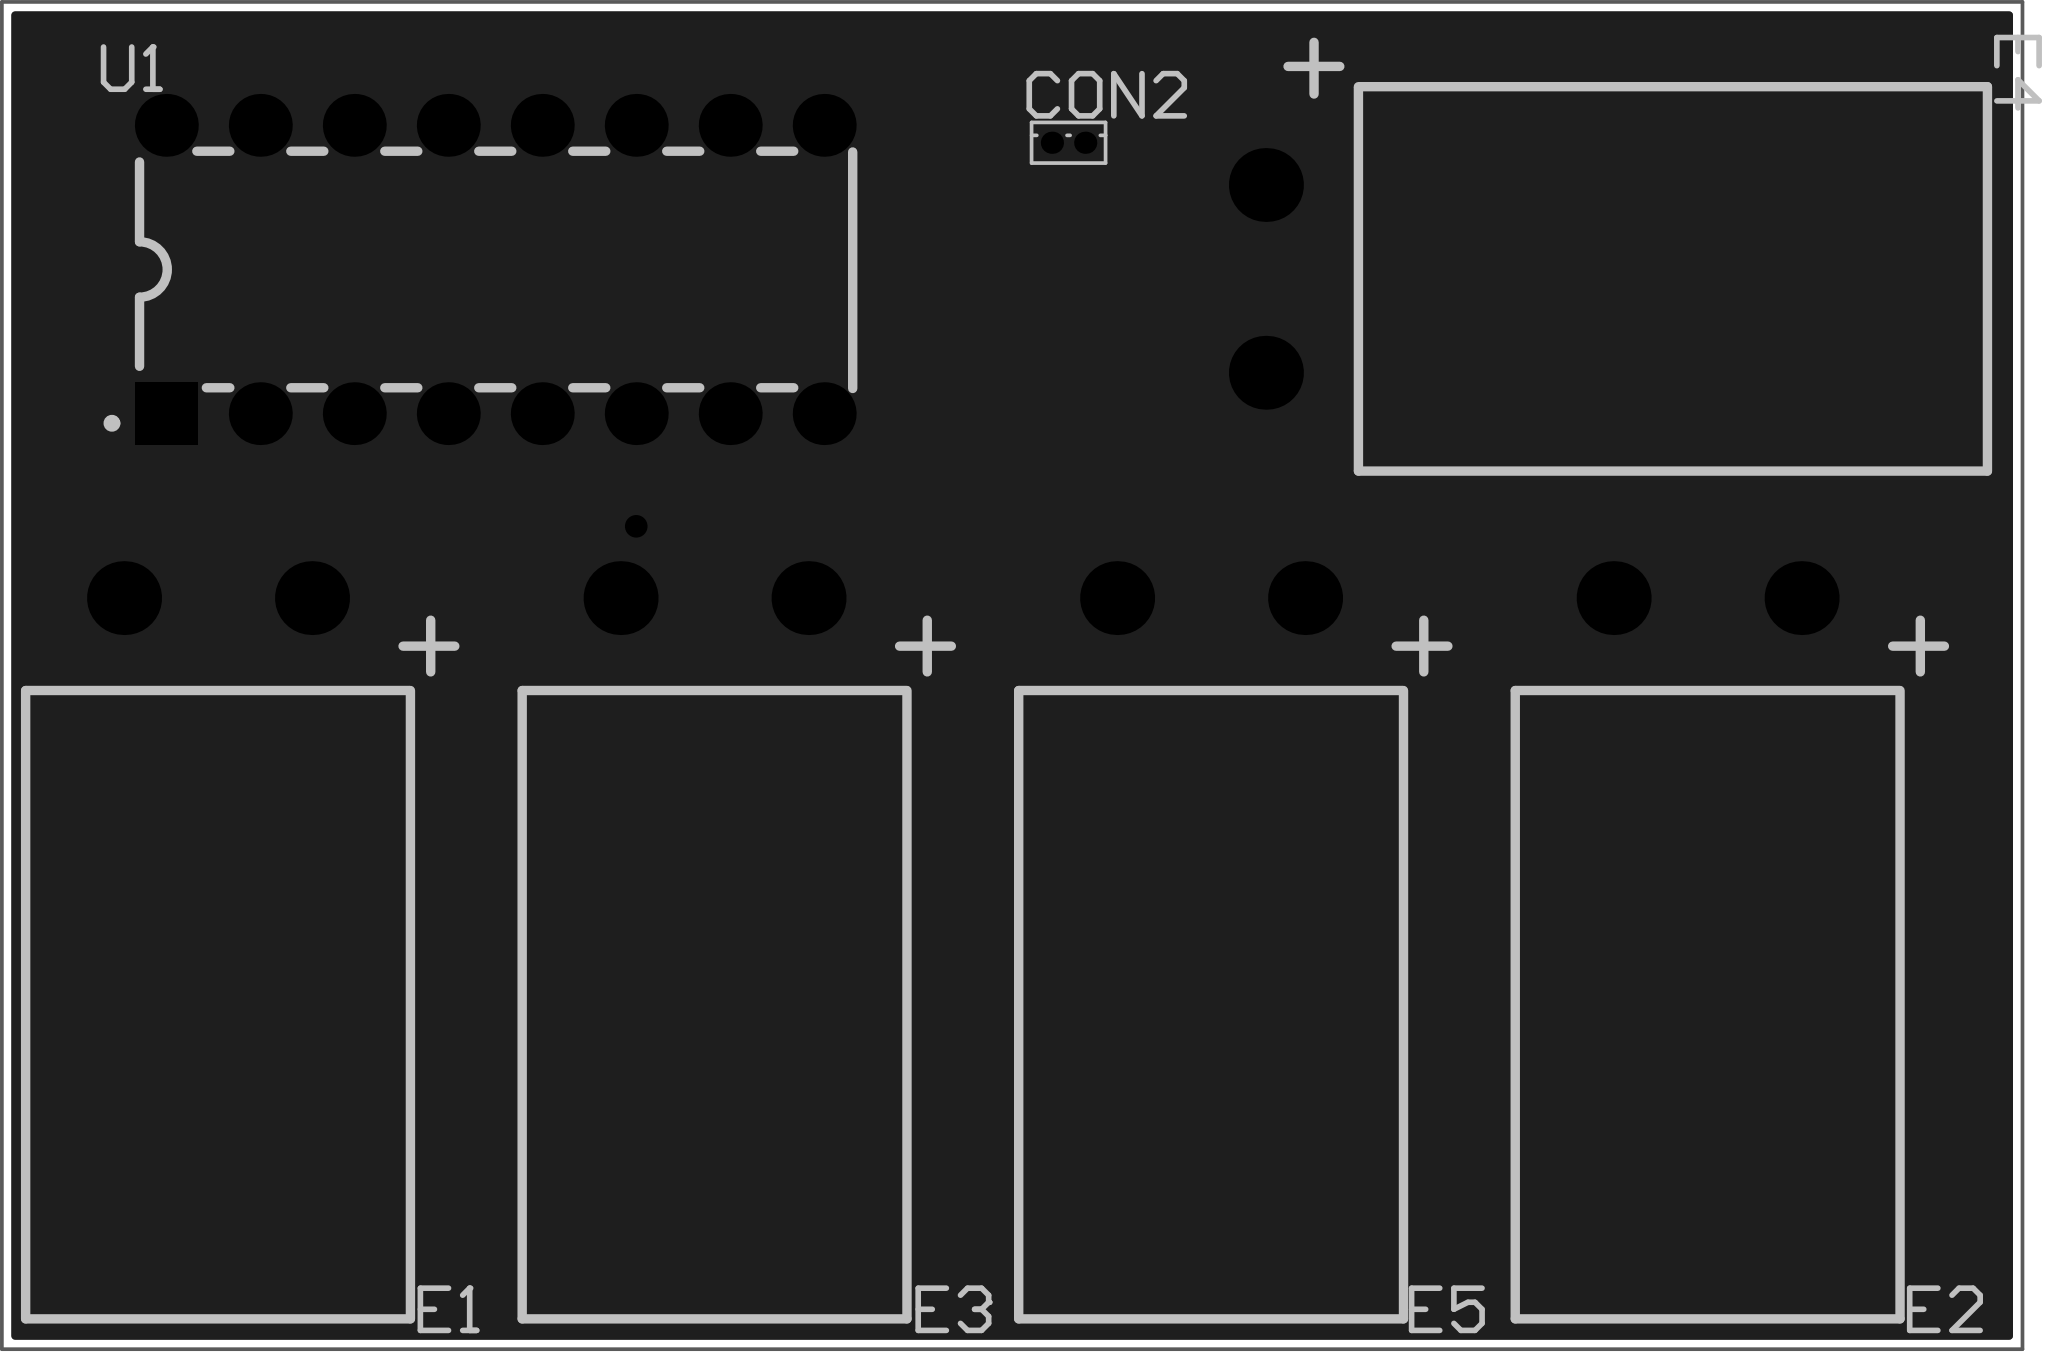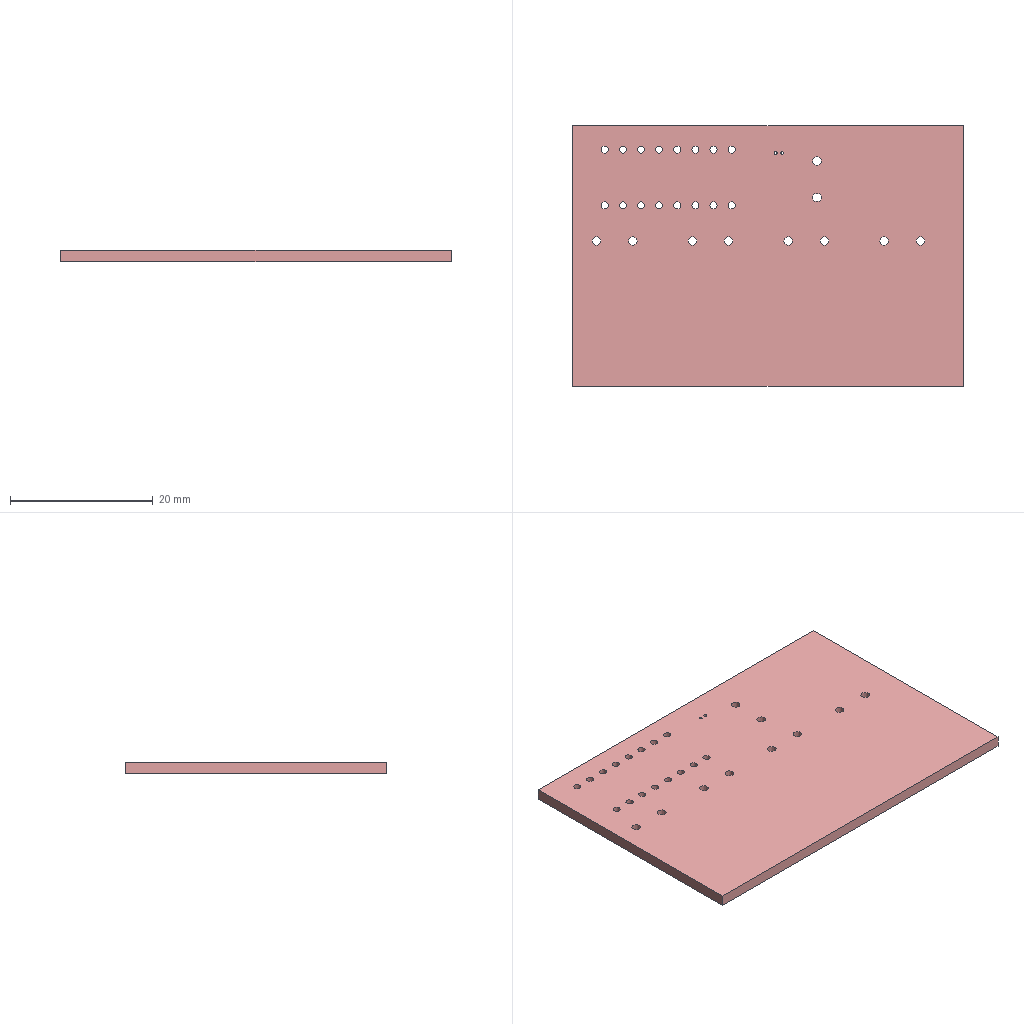Circuit board layout | Altium Designer | box 54.6 x 36.4 x 1.6 mm
Layer stack:
# Altium Designer layer stack of  (unit mm; dielectric type: 0 none, 1 core, 2 prepreg, 3 surface material)
index,name,kind,layer,copper_thickness_mm,dielectric_type,dielectric_thickness_mm,dielectric_material,dielectric_constant
0,Top Paste Mask Layer,other,,,,,,
1,Top Silkscreen Layer,other,,,,,,
2,Top Solder Mask Layer,dielectric,,,3,0.01,,3.3
3,Top Layer,copper,Top Layer,0.035,,,,
4,Dielectric1,dielectric,,,3,1.51,FR4,4.5
5,Bottom Layer,copper,Bottom Layer,0.035,,,,
6,Bottom Solder Mask Layer,dielectric,,,3,0.01,,3.3
7,Bottom Silkscreen Layer,other,,,,,,
8,Bottom Paste Mask Layer,other,,,,,,
# drill layer pairs: low layer,high layer
drill_pair,Top Layer,Bottom Layer
Part placement:
Designator,Comment,Layer,Footprint,Center-X(mm),Center-Y(mm),Rotation
CON2,,TopLayer,SIP-2_L2.0-W1.1-P0.90-D0.3,106.553,109.601,0
E1,1uf,TopLayer,CAP-TH_L17.0-W10.4-P5.08_CDK11A_470UF,83.566,97.282,180
E2,1uf,TopLayer,CAP-TH_L17.0-W10.4-P5.08_CDK11A_470UF,123.825,97.282,180
E3,1uf,TopLayer,CAP-TH_L17.0-W10.4-P5.08_CDK11A_470UF,96.986,97.282,180
E4,1uf,TopLayer,CAP-TH_L17.0-W10.4-P5.08_CDK11A_470UF,111.887,105.918,270
E5,1uf,TopLayer,CAP-TH_L17.0-W10.4-P5.08_CDK11A_470UF,110.405,97.282,180
U1,MAX232IDR-TD,TopLayer,DIP-16_L19.7-W6.6-P2.54-LS10.9-BL,91.059,106.172,0
Pad and via stacks:
# Altium Designer via and pad stacks of  (unit mm). Each distinct definition once, with the count of objects using it.
# via: kind,start_layer,end_layer,hole_mm,diameter_mm,mode(0 simple;1 top-mid-bottom;2 full stack),diameter_per_layer,count,example_net
# pad: kind,layer,hole_mm,hole_type(0 round;1 square;2 slot),plating,top_size,top_shape(1 round;2 rect;3 octagon;9 rounded rect),mid_size,bottom_size,mode,footprint,size_per_layer,count,example
pad,Multi-Layer,0.4,0,plated,0.6x0.6,1,0.6x0.6,0.6x0.6,0,SIP-2_L2.0-W1.1-P0.90-D0.3,,2,CON2.1
pad,Multi-Layer,1.2,0,plated,2x2,1,2x2,2x2,0,CAP-TH_L17.0-W10.4-P5.08_CDK11A_470UF,,10,E1.1
pad,Multi-Layer,1,0,plated,1.7x1.7,2,1.7x1.7,1.7x1.7,0,DIP-16_L19.7-W6.6-P2.54-LS10.9-BL,,1,U1.1
pad,Multi-Layer,1,0,plated,1.7x1.7,1,1.7x1.7,1.7x1.7,0,DIP-16_L19.7-W6.6-P2.54-LS10.9-BL,,15,U1.2
via,Top Layer,Bottom Layer,0.3048,0.61,0,,1,$1N627
Copper pours:
name,layer,net,type(0 solid;1 hatched;2 none)
Top Layer-GND,Top Layer,GND,0
Bottom Layer-GND,Bottom Layer,GND,0
Design rules, without the lines most boards share:
# Altium Designer design rules of  (exported by Altium Designer, unit mm)
# columns: name | kind | enabled | priority | scope1 | scope2 | descriptor | typed fields (field=value)
copperThickness1oz_2 | 2 | enabled | 2 | All | All | Width Constraint (Min=5mil) (Max=100mil) (Preferred=30mil) (All) |
viaSize | 11 | enabled | 1 | All | All | Routing Via (MinHoleWidth=11.811mil) (MaxHoleWidth=248.032mil) (PreferredHoleWidth=12.008mil) (MinWidth=19.685mil) (MaxWidth=393.701mil) (PreferedWidth=24.016mil) (All) | via_min_hole=0.3 via_max_hole=6.3 via_preferred_diameter=0.61 via_preferred_hole=0.305
solderMaskExpansion | 13 | enabled | 2 | All | All | Solder Mask Expansion (Expansion =2.008mil) (All) | expansion=0.051